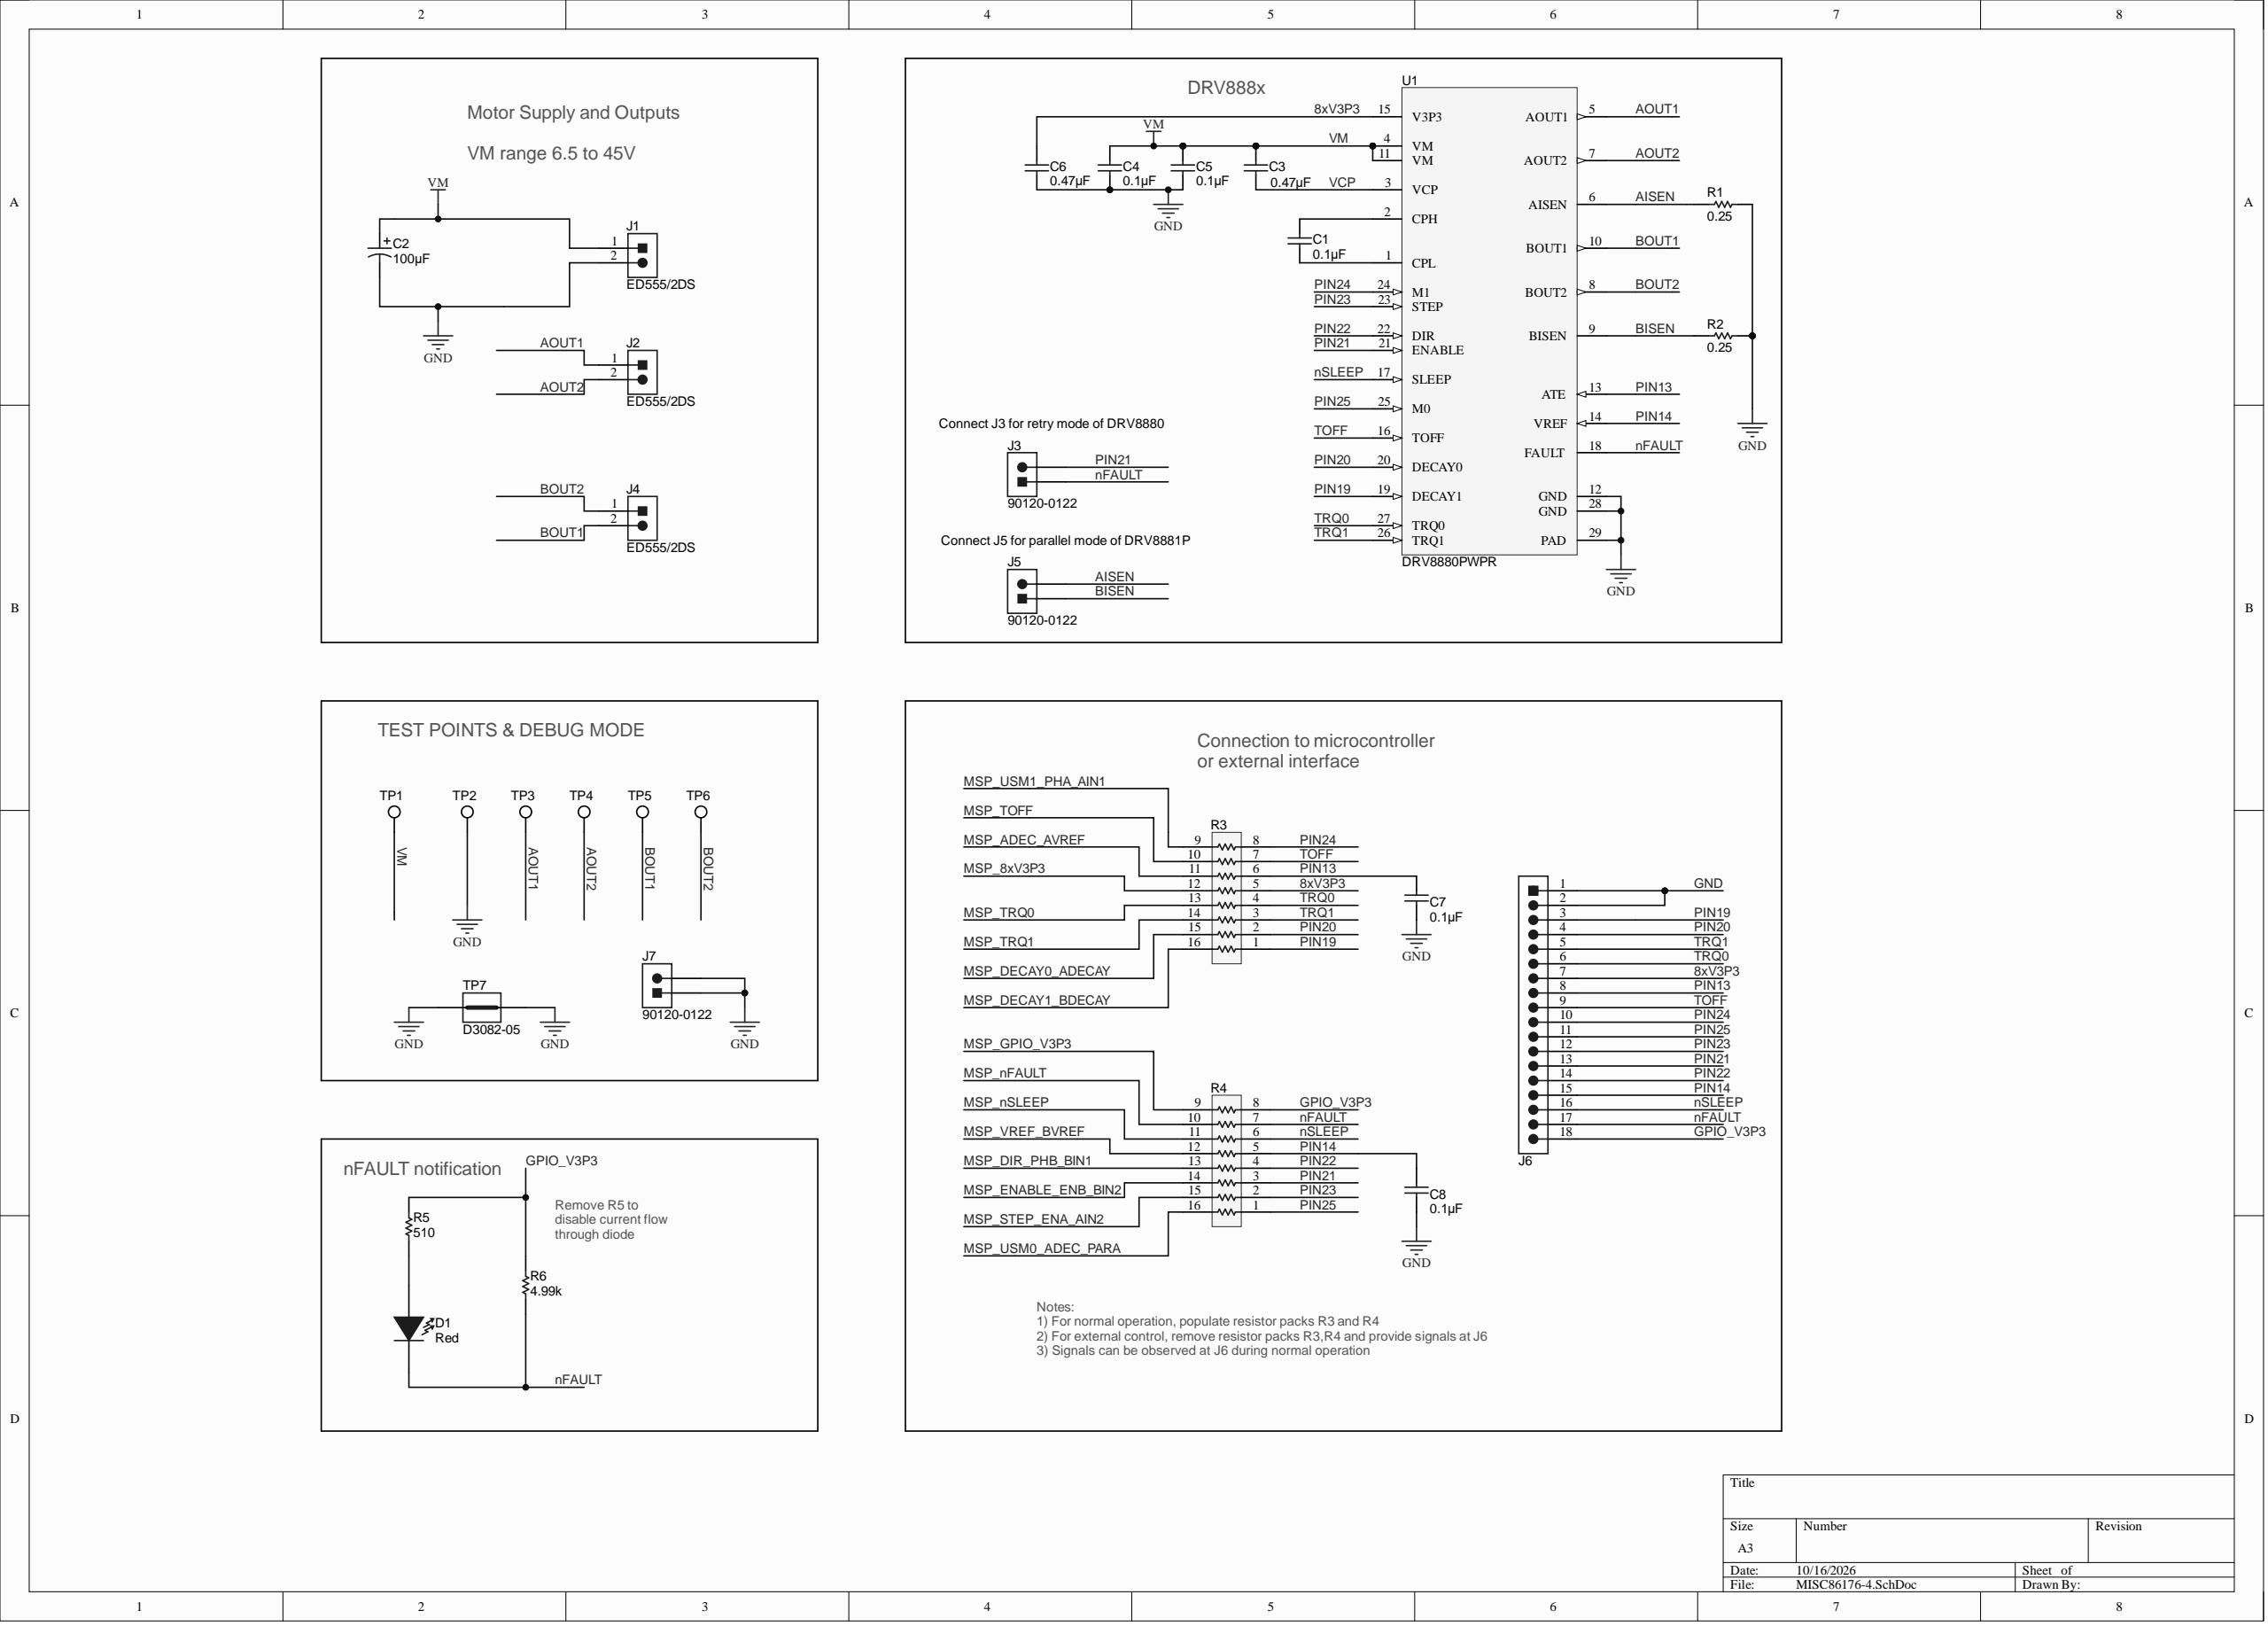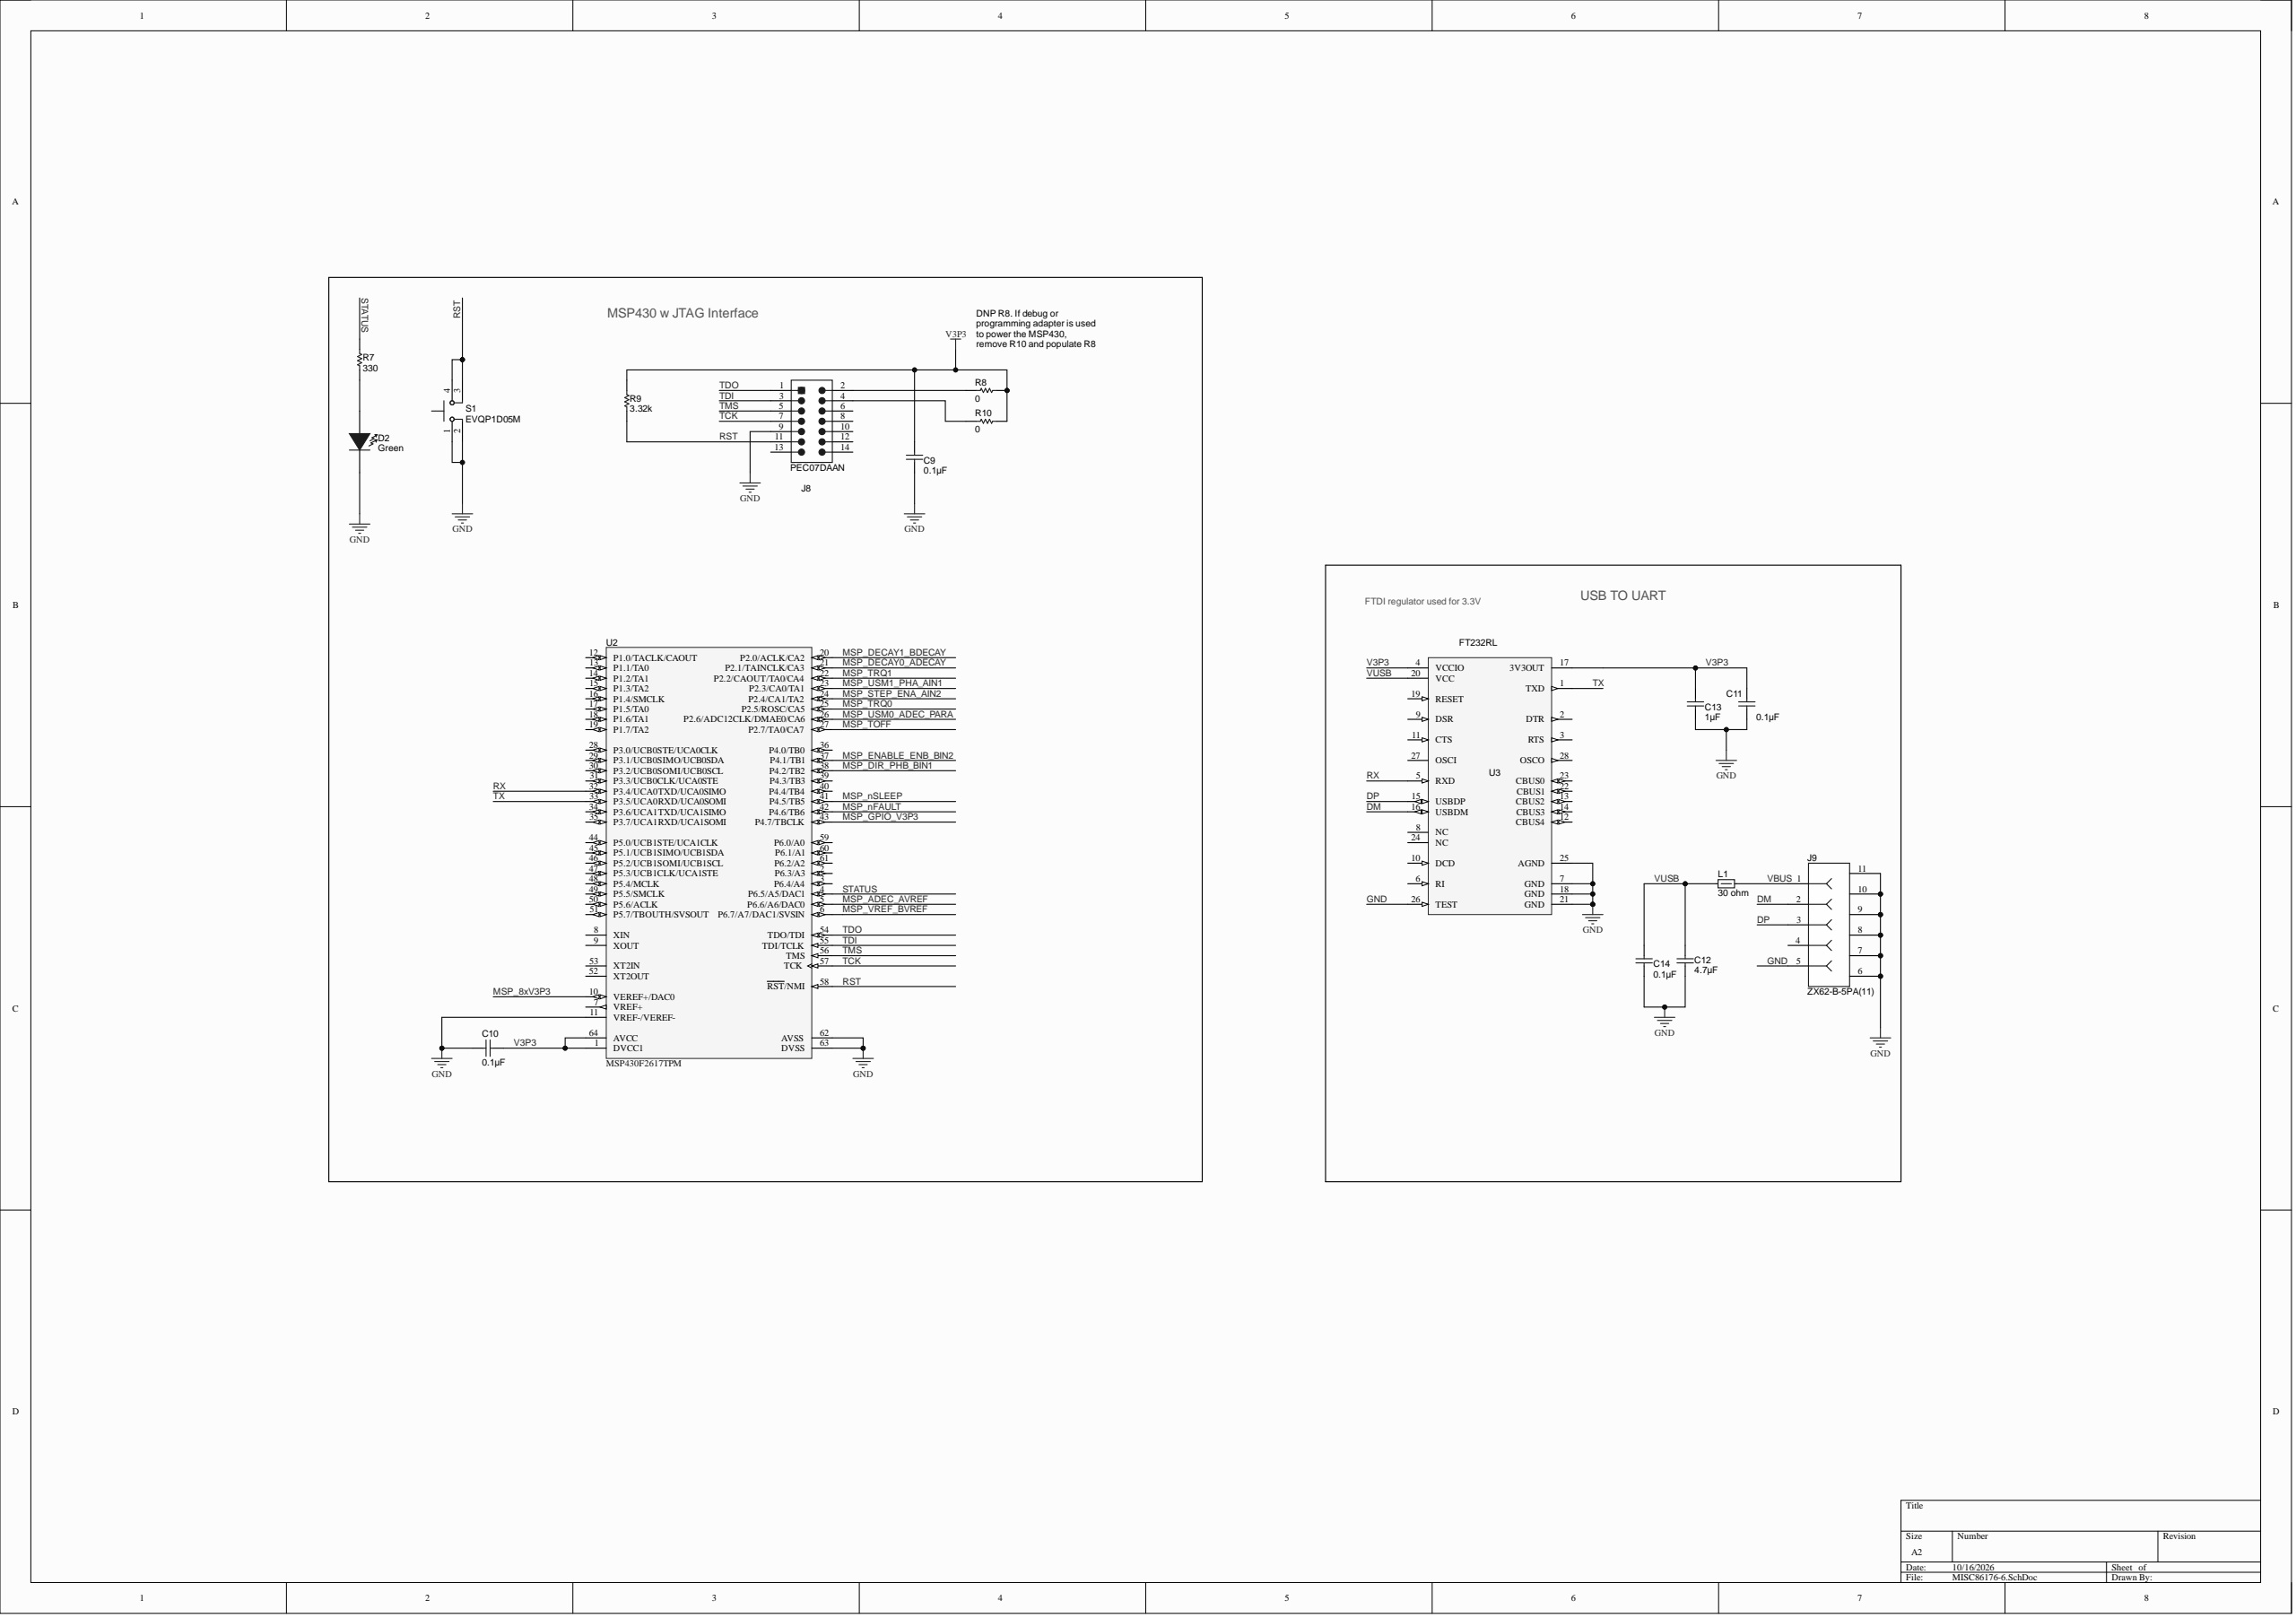Circuit board | Altium Designer | 47 parts | 60 nets
Bill of materials:
Comment,Description,Designator,Footprint,LibRef,Quantity
"C0805C104K1RACTU","CAP, CERM, 0.1 µF, 100 V, +/- 10%, X7R, 0805","C1, C4, C5","0805L","C0805C104K1RACTU","3"
"EEE-FK1J101P","CAP, AL, 100 µF, 63 V, +/- 20%, 0.35 ohm, SMD","C2","SM_RADIAL_G","EEE-FK1J101P","1"
"C2012X7R1E474K","CAP, CERM, 0.47 µF, 25 V, +/- 10%, X7R, 0805","C3","0805L","C2012X7R1E474K","1"
"C0603C474K9RACTU","CAP, CERM, 0.47 µF, 6.3 V, +/- 10%, X7R, 0603","C6","0603L","C0603C474K9RACTU","1"
"GRM155R61A104KA01D","CAP, CERM, 0.1 µF, 10 V, +/- 10%, X5R, 0402","C7, C8, C9, C10, C11, C14","0402L","GRM155R61A104KA01D","6"
"CGB3B1X5R1A475K055AC","CAP, CERM, 4.7 µF, 10 V, +/- 10%, X5R, 0603","C12","0603L","CGB3B1X5R1A475K055AC","1"
"GRM155R61A105KE15D","CAP, CERM, 1 µF, 10 V, +/- 10%, X5R, 0402","C13","0402L","GRM155R61A105KE15D","1"
"LTST-C190CKT","LED, Red, SMD","D1","LED_LTST-C190_Red","LTST-C190CKT","1"
"LTST-C190GKT","LED, Green, SMD","D2","LED_LTST-C190","LTST-C190GKT","1"
"ED555/2DS","Terminal Block, 6A, 3.5mm Pitch, 2-Pos, TH","J1, J2, J4","TERM_BLK_ED555-2DS","ED555/2DS","3"
"90120-0122","Header, 100mil, 2x1, Tin, TH","J3, J5, J7","CONN_90120-0122","90120-0122","3"
"TSW-118-07-G-S","Header, 100mil, 18x1, Gold, TH","J6","TSW-118-07-G-S","TSW-118-07-G-S","1"
"PEC07DAAN","Header, 100mil, 7x2, Tin, TH","J8","CONN_PEC07DAAN","PEC07DAAN","1"
"ZX62-B-5PA(11)","Connector, Receptacle, Micro-USB Type B, R/A, Bottom Mount SMT","J9","CONN_USB_micro_ZX62-B-5PA","ZX62-B-5PA(11)","1"
"MMZ2012R300A","Ferrite Bead, 30 ohm @ 100 MHz, 1.5 A, 0805","L1","0805L","MMZ2012R300A","1"
"CSRN2010FKR250","RES, 0.25, 1%, 1 W, 2010","R1, R2","2010L","CSRN2010FKR250","2"
"EXB-2HV330JV","RES, 33, 5%, 0.0625 W, Resistor Array - 8x1","R3, R4","RESCAXS_EXB-2HV","EXB-2HV330JV","2"
"CRCW0402510RJNED","RES, 510, 5%, 0.063 W, 0402","R5","0402L","CRCW0402510RJNED","1"
"CRCW04024K99FKED","RES, 4.99 k, 1%, 0.063 W, 0402","R6","0402L","CRCW04024K99FKED","1"
"CRCW0402330RJNED","RES, 330, 5%, 0.063 W, 0402","R7","0402L","CRCW0402330RJNED","1"
"ERJ-2GE0R00X","RES, 0, 5%, 0.063 W, 0402","R8, R10","0402L","ERJ-2GE0R00X","2"
"CRCW04023K32FKED","RES, 3.32 k, 1%, 0.063 W, 0402","R9","0402L","CRCW04023K32FKED","1"
"EVQP1D05M","Switch, Tactile, SPST-NO, 0.05A, 12V, SMT","S1","SW_EVQxxx05M","EVQP1D05M","1"
"5016","Test Point, Compact, SMT","TP1, TP2, TP3, TP4, TP5, TP6","Testpoint_Keystone_Compact","5016","6"
"D3082-05","1mm Uninsulated Shorting Plug, 10.16mm spacing, TH","TP7","Harwin_D3082-05","D3082-05","1"
"DRV8880PWPR","2-A 45-V 1/16-µstep Stepper Motor Driver With AutoTune, PWP0028C","U1","PWP0028C_N","DRV8880PWPR","1"
"MSP430F2617TPM","16 MHz Mixed Signal Microcontroller with 92 KB Flash, 8192 B SRAM and 48 GPIOs, -40 to 105 degC, 64-pin QFP (PM), Green (RoHS & no Sb/Br)","U2","PM0064A_L","MSP430F2617TPM","1"
"FT232RL","USB to Serial UART, SSOP28","U3","SSOP28_M","FT232RL","1"
Netlist (Protel format):
[
C1
0805L
C0805C104K1RACTU



]
[
C2
SM_RADIAL_G
EEE-FK1J101P



]
[
C3
0805L
C2012X7R1E474K



]
[
C4
0805L
C0805C104K1RACTU



]
[
C5
0805L
C0805C104K1RACTU



]
[
C6
0603L
C0603C474K9RACTU



]
[
C7
0402L
GRM155R61A104KA01D



]
[
C8
0402L
GRM155R61A104KA01D



]
[
C9
0402L
GRM155R61A104KA01D



]
[
C10
0402L
GRM155R61A104KA01D



]
[
C11
0402L
GRM155R61A104KA01D



]
[
C12
0603L
CGB3B1X5R1A475K055AC



]
[
C13
0402L
GRM155R61A105KE15D



]
[
C14
0402L
GRM155R61A104KA01D



]
[
D1
LED_LTST-C190_Red
LTST-C190CKT



]
[
D2
LED_LTST-C190
LTST-C190GKT



]
[
J1
TERM_BLK_ED555-2DS
ED555/2DS



]
[
J2
TERM_BLK_ED555-2DS
ED555/2DS



]
[
J3
CONN_90120-0122
90120-0122



]
[
J4
TERM_BLK_ED555-2DS
ED555/2DS



]
[
J5
CONN_90120-0122
90120-0122



]
[
J6
TSW-118-07-G-S
TSW-118-07-G-S



]
[
J7
CONN_90120-0122
90120-0122



]
[
J8
CONN_PEC07DAAN
PEC07DAAN



]
[
J9
CONN_USB_micro_ZX62-B-5PA
ZX62-B-5PA(11)



]
[
L1
0805L
MMZ2012R300A



]
[
R1
2010L
CSRN2010FKR250



]
[
R2
2010L
CSRN2010FKR250



]
[
R3
RESCAXS_EXB-2HV
EXB-2HV330JV



]
[
R4
RESCAXS_EXB-2HV
EXB-2HV330JV



]
[
R5
0402L
CRCW0402510RJNED



]
[
R6
0402L
CRCW04024K99FKED



]
[
R7
0402L
CRCW0402330RJNED



]
[
R8
0402L
ERJ-2GE0R00X



]
[
R9
0402L
CRCW04023K32FKED



]
[
R10
0402L
ERJ-2GE0R00X



]
[
S1
SW_EVQxxx05M
EVQP1D05M



]
[
TP1
Testpoint_Keystone_Compact
5016



]
[
TP2
Testpoint_Keystone_Compact
5016



]
[
TP3
Testpoint_Keystone_Compact
5016



]
[
TP4
Testpoint_Keystone_Compact
5016



]
[
TP5
Testpoint_Keystone_Compact
5016



]
[
TP6
Testpoint_Keystone_Compact
5016



]
[
TP7
Harwin_D3082-05
D3082-05



]
[
U1
PWP0028C_N
DRV8880PWPR



]
[
U2
PM0064A_L
MSP430F2617TPM



]
[
U3
SSOP28_M
FT232RL



]
(
VUSB
C12-1
C14-1
L1-1
U3-20
)
(
VM
C2-1
C3-2
C4-2
C5-2
J1-1
TP1-1
U1-4
U1-11
)
(
VCP
C3-1
U1-3
)
(
VBUS
J9-1
L1-2
)
(
V3P3
C9-1
C10-1
C11-1
C13-1
R8-1
R9-2
R10-1
U2-1
U2-64
U3-4
U3-17
)
(
TX
U2-33
U3-1
)
(
TRQ1
J6-5
R3-3
U1-26
)
(
TRQ0
J6-6
R3-4
U1-27
)
(
TOFF
J6-9
R3-7
U1-16
)
(
TMS
J8-5
U2-56
)
(
TDO
J8-1
U2-54
)
(
TDI
J8-3
U2-55
)
(
TCK
J8-7
U2-57
)
(
STATUS
R7-2
U2-4
)
(
RX
U2-32
U3-5
)
(
RST
J8-11
R9-1
S1-3
S1-4
U2-58
)
(
PIN25
J6-11
R4-1
U1-25
)
(
PIN24
J6-10
R3-8
U1-24
)
(
PIN23
J6-12
R4-2
U1-23
)
(
PIN22
J6-14
R4-4
U1-22
)
(
PIN21
J3-2
J6-13
R4-3
U1-21
)
(
PIN20
J6-4
R3-2
U1-20
)
(
PIN19
J6-3
R3-1
U1-19
)
(
PIN14
C8-1
J6-15
R4-5
U1-14
)
(
PIN13
C7-1
J6-8
R3-6
U1-13
)
(
nSLEEP
J6-16
R4-6
U1-17
)
(
nFAULT
D1-2
J3-1
J6-17
R4-7
R6-1
U1-18
)
(
NetJ8_4
J8-4
R10-2
)
(
NetJ8_2
J8-2
R8-2
)
(
NetD2_1
D2-1
R7-1
)
(
NetD1_1
D1-1
R5-1
)
(
NetC1_2
C1-2
U1-2
)
(
NetC1_1
C1-1
U1-1
)
(
MSP_VREF_BVREF
R4-12
U2-6
)
(
MSP_USM1_PHA_AIN1
R3-9
U2-23
)
(
MSP_USM0_ADEC_PARA
R4-16
U2-26
)
(
MSP_TRQ1
R3-14
U2-22
)
(
MSP_TRQ0
R3-13
U2-25
)
(
MSP_TOFF
R3-10
U2-27
)
(
MSP_STEP_ENA_AIN2
R4-15
U2-24
)
(
MSP_nSLEEP
R4-11
U2-41
)
(
MSP_nFAULT
R4-10
U2-42
)
(
MSP_GPIO_V3P3
R4-9
U2-43
)
(
MSP_ENABLE_ENB_BIN2
R4-14
U2-37
)
(
MSP_DIR_PHB_BIN1
R4-13
U2-38
)
(
MSP_DECAY1_BDECAY
R3-16
U2-20
)
(
MSP_DECAY0_ADECAY
R3-15
U2-21
)
(
MSP_ADEC_AVREF
R3-11
U2-5
)
(
MSP_8xV3P3
R3-12
U2-10
)
(
GPIO_V3P3
J6-18
R4-8
R5-2
R6-2
)
(
GND
C2-2
C4-1
C5-1
C6-2
C7-2
C8-2
C9-2
C10-2
C11-2
C12-2
C13-2
C14-2
D2-2
J1-2
J6-1
J6-2
J7-1
J7-2
J8-9
J9-5
J9-6
J9-7
J9-8
J9-9
J9-10
J9-11
R1-1
R2-1
S1-1
S1-2
TP2-1
TP7-1
TP7-2
U1-12
U1-28
U1-29
U2-11
U2-62
U2-63
U3-7
U3-18
U3-21
U3-25
U3-26
)
(
DP
J9-3
U3-15
)
(
DM
J9-2
U3-16
)
(
BOUT2
J4-1
TP6-1
U1-8
)
(
BOUT1
J4-2
TP5-1
U1-10
)
(
BISEN
J5-1
R2-2
U1-9
)
(
AOUT2
J2-2
TP4-1
U1-7
)
(
AOUT1
J2-1
TP3-1
U1-5
)
(
AISEN
J5-2
R1-2
U1-6
)
(
8xV3P3
C6-1
J6-7
R3-5
U1-15
)